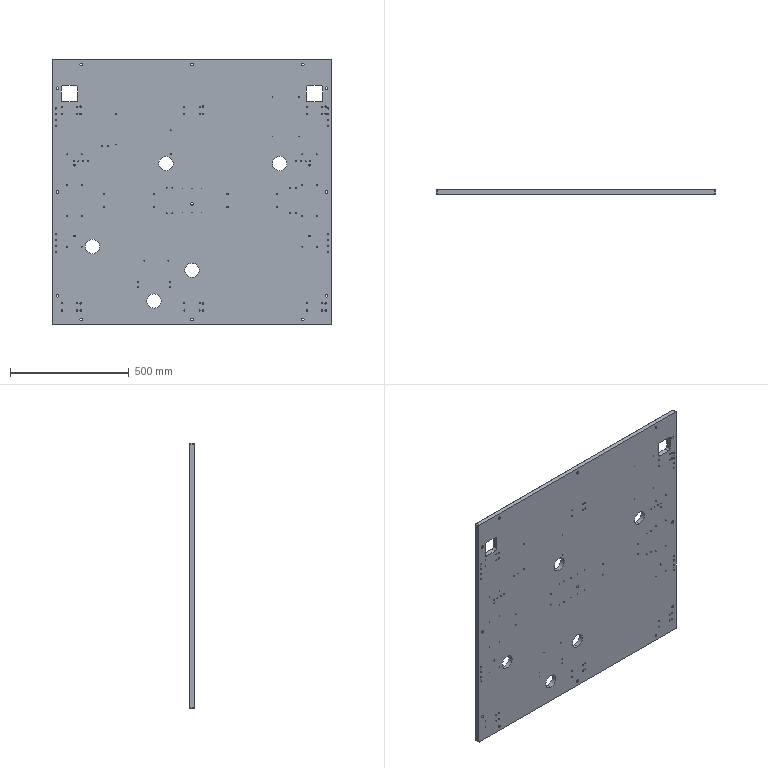Part | STEP file | 1 solid | 513 faces | box 1180 x 20 x 1120 mm | volume 25848378 mm3 | cylinder 406 | plane 55 | cone 52 | commonest cylinder face diameters 5 x96 3.3 x76 4.2 x64 6 x48 8 x32 11 x26